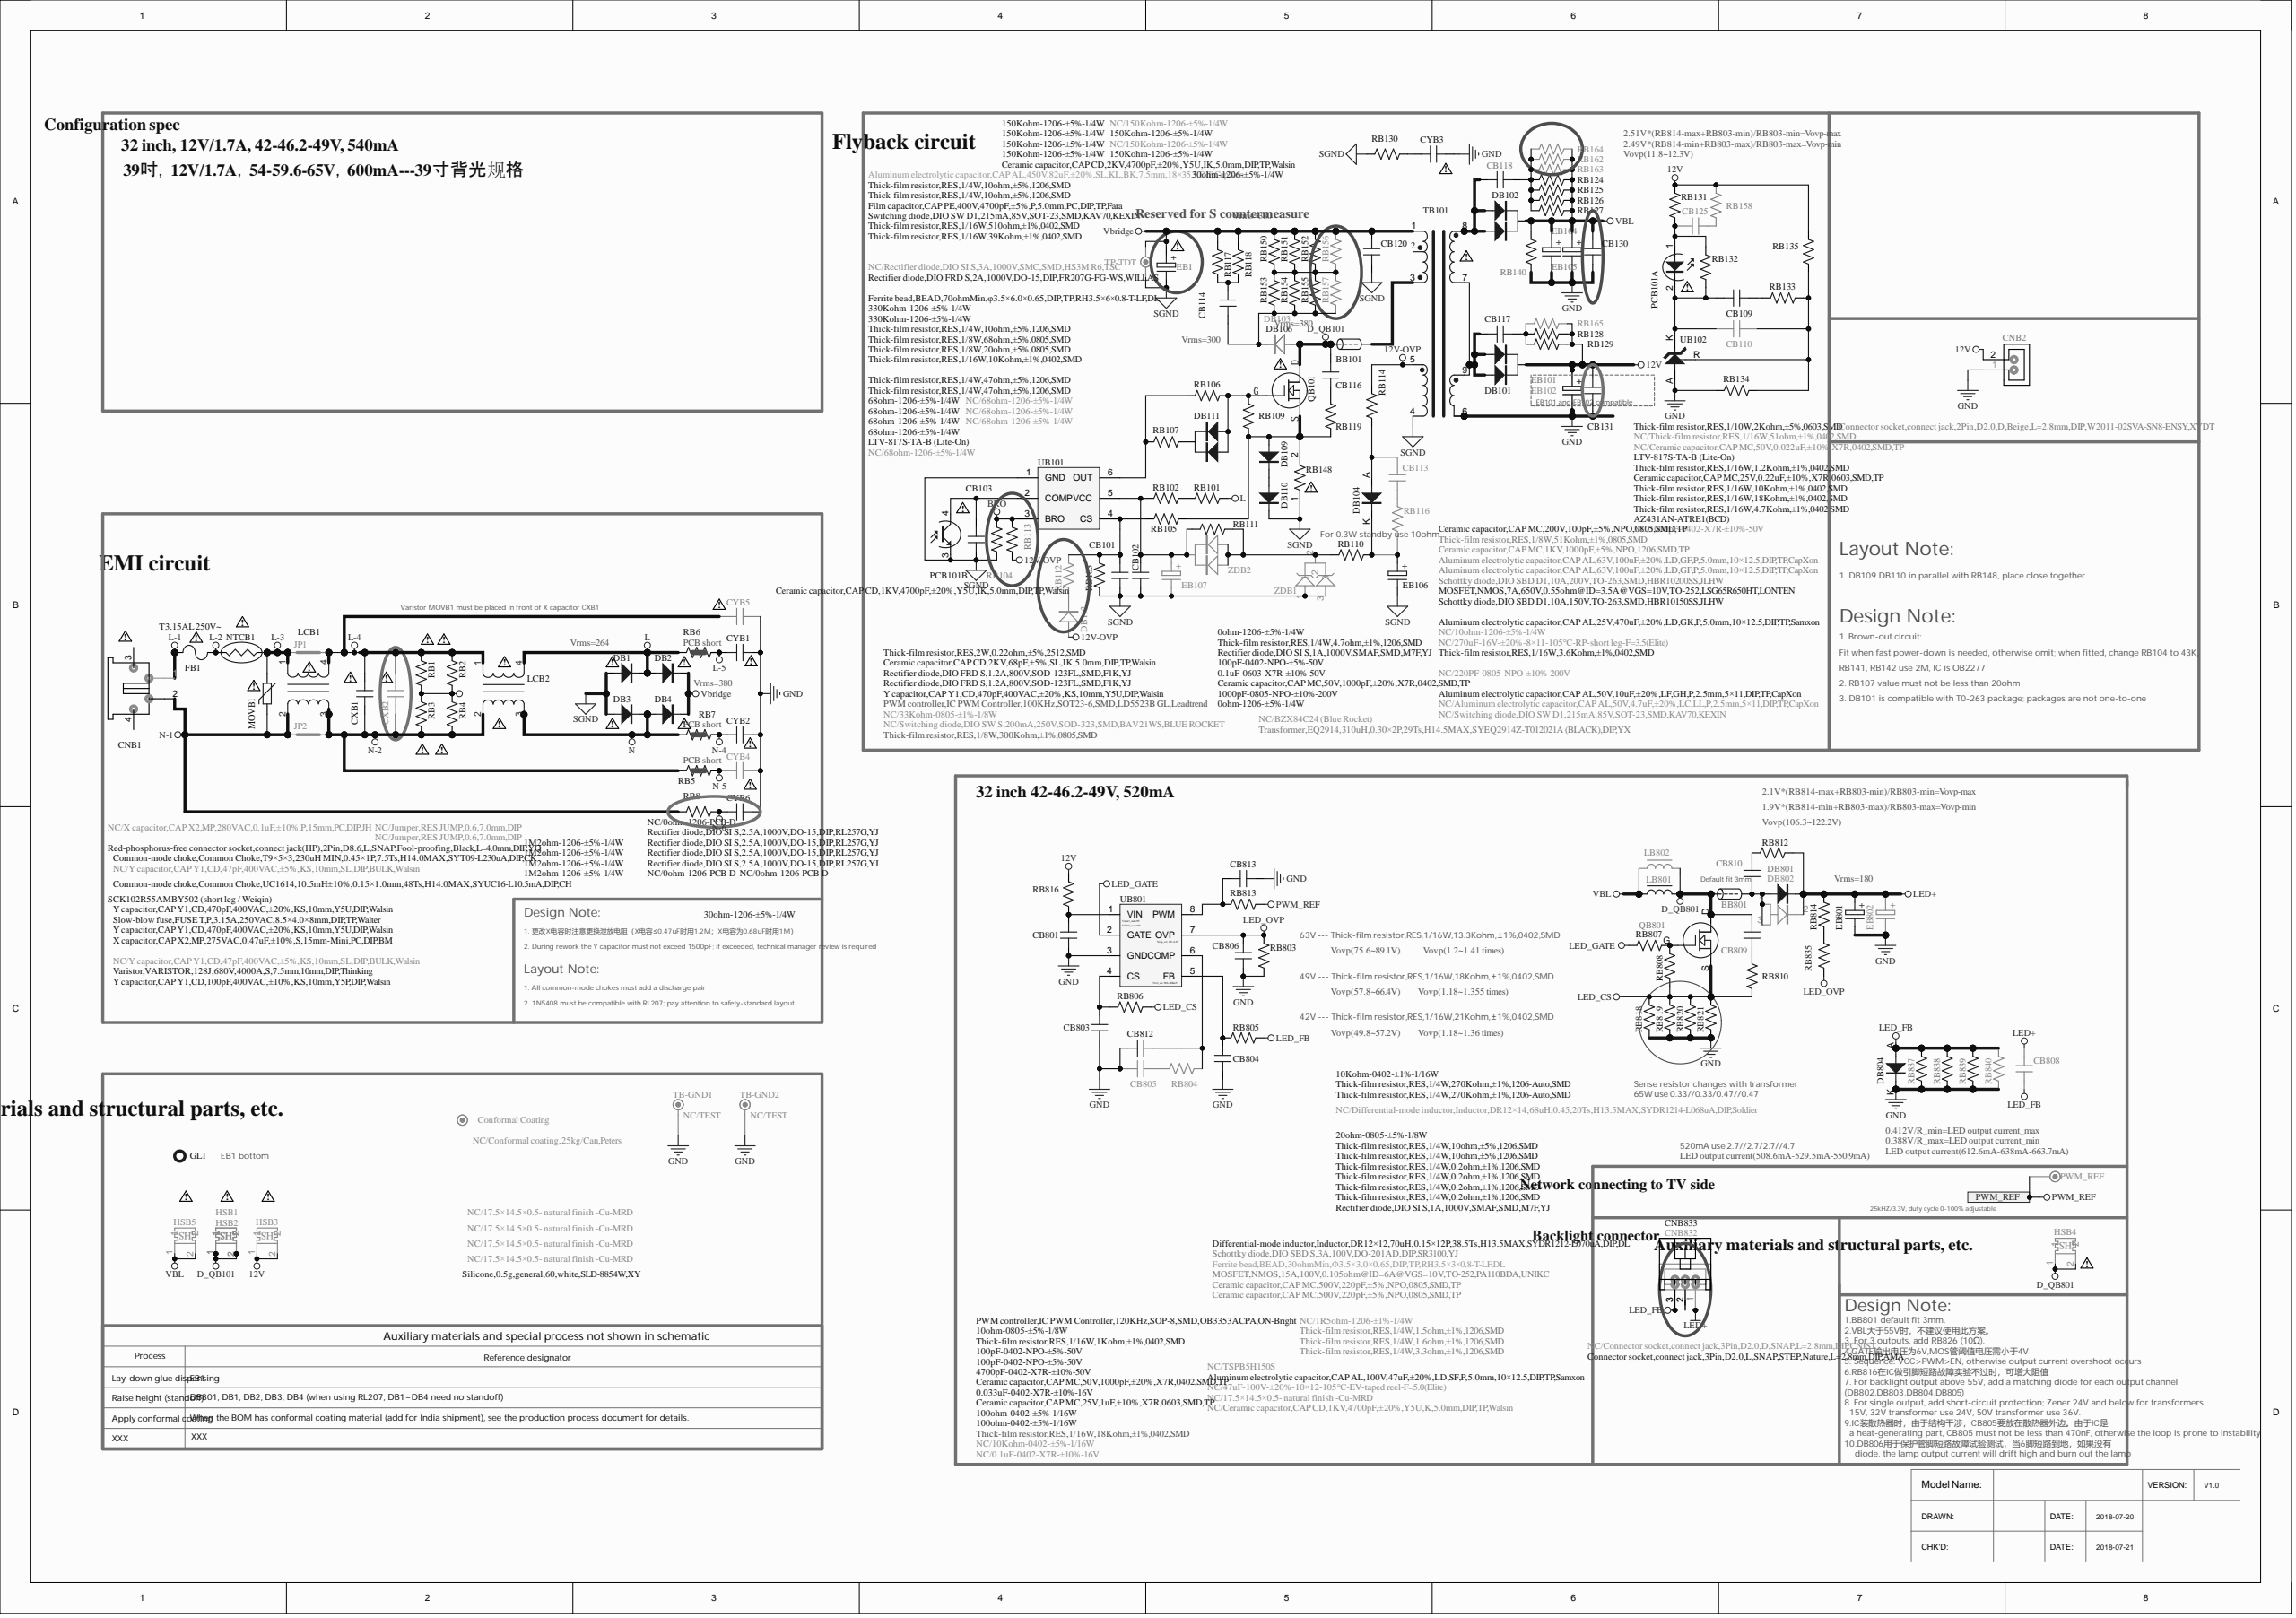Circuit board | Altium Designer | 574 parts | 274 nets | one sheet of the schematic
Parts on this sheet (reference | value | footprint):
BB101 | Ferrite bead,BEAD,70ohmMin,f3.5×6.0×0.65,DIP,TP,RH3.5×6×0.8-T-LF,DL | LB/3.5*6*12.5
BB801 | Ferrite bead,BEAD,30ohmMin,F3.5×3.0×0.65,DIP,TP,RH3.5×3×0.8-T-LF,DL | LB/3.5*6*12.5
CB101 | 100pF-0402-NPO-±5%-50V | C0402
CB102 | 0.1uF-0603-X7R-±10%-50V | C0603
CB103 | Ceramic capacitor,CAP MC,50V,1000pF,±20%,X7R,0402,SMD,TP | C0402
CB109 | Ceramic capacitor,CAP MC,25V,0.22uF,±10%,X7R,0603,SMD,TP | C0603
CB110 | NC/1000pF-0402-X7R-±10%-50V | C0402
CB113 | NC/220PF-0805-NPO-±10%-200V | C0805
CB114 | Film capacitor,CAP PE,400V,4700pF,±5%,P,5.0mm,PC,DIP,TP,Fara | CAP8*2.5-V-5
CB116 | Ceramic capacitor,CAP CD,2KV,68pF,±5%,SL,IK,5.0mm,DIP,TP,Walsin | CAP6.5*5-V-5-1
CB117 | 1000pF-0805-NPO-±10%-200V | C0805
CB118 | Ceramic capacitor,CAP MC,1KV,1000pF,±5%,NPO,1206,SMD,TP | C1206
CB120 | Ceramic capacitor,CAP CD,2KV,4700pF,±20%,Y5U,IK,5.0mm,DIP,TP,Walsin | CAP10*4.5-V-5
CB125 | NC/Ceramic capacitor,CAP MC,50V,0.022uF,±10%,X7R,0402,SMD,TP | C0402
CB130 | Ceramic capacitor,CAP CD,1KV,4700pF,±20%,Y5U,IK,5.0mm,DIP,TP,Walsin | CAP10*4.5-V-5
CB131 | Ceramic capacitor,CAP MC,200V,100pF,±5%,NPO,0805,SMD,TP | C0805
CB801 | Ceramic capacitor,CAP MC,25V,1uF,±10%,X7R,0603,SMD,TP | C0603
CB803 | 100pF-0402-NPO-±5%-50V | C0402
CB804 | 4700pF-0402-X7R-±10%-50V | C0402
CB805 | NC/0.1uF-0402-X7R-±10%-16V | C0402
CB806 | Ceramic capacitor,CAP MC,50V,1000pF,±20%,X7R,0402,SMD,TP | C0402
CB808 | NC/Ceramic capacitor,CAP CD,1KV,4700pF,±20%,Y5U,K,5.0mm,DIP,TP,Walsin | CAP10*4.5-V-5
CB809 | Ceramic capacitor,CAP MC,500V,220pF,±5%,NPO,0805,SMD,TP | C0805
CB810 | Ceramic capacitor,CAP MC,500V,220pF,±5%,NPO,0805,SMD,TP | C0805
CB812 | 0.033uF-0402-X7R-±10%-16V | C0402
CB813 | 100pF-0402-NPO-±5%-50V | C0402
CNB1 | Red-phosphorus-free connector socket,connect jack(HP),2Pin,D8.6,L,SNAP,Fool-proofing,Black,L=4.0mm,DIP,YQ | CON2-H8.6-1
CNB2 | Connector socket,connect jack,2Pin,D2.0,D,Beige,L=2.8mm,DIP,W2011-02SVA-SN8-ENSY,XYDT | SIP2/2.0D-1
CNB832 | NC/Connector socket,connect jack,3Pin,D2.0,D,SNAP,L=2.8mm,DIP,CNJST | SIP3/2.0D-CP
CNB833 | Connector socket,connect jack,3Pin,D2.0,L,SNAP,STEP,Nature,L=2.8mm,DIP,AMA | SIP3H/2.0D-3
CXB1 | X capacitor,CAP X2,MP,275VAC,0.47uF,±10%,S,15mm-Mini,PC,DIP,BM | CAP18*8.5-V-15
CXB2 | NC/X capacitor,CAP X2,MP,280VAC,0.1uF,±10%,P,15mm,PC,DIP,JH | CAP18*5*11.5-V-15
CYB1 | Y capacitor,CAP Y1,CD,470pF,400VAC,±20%,KS,10mm,Y5U,DIP,Walsin | CAP13*5-V-10-1
CYB2 | Y capacitor,CAP Y1,CD,470pF,400VAC,±20%,KS,10mm,Y5U,DIP,Walsin | CAP13*5-V-10-1
CYB3 | Y capacitor,CAP Y1,CD,470pF,400VAC,±20%,KS,10mm,Y5U,DIP,Walsin | CAP13*5-V-10-1
CYB4 | NC/Y capacitor,CAP Y1,CD,47pF,400VAC,±5%,KS,10mm,SL,DIP,BULK,Walsin | CAP13*5-V-10-1
CYB5 | NC/Y capacitor,CAP Y1,CD,47pF,400VAC,±5%,KS,10mm,SL,DIP,BULK,Walsin | CAP13*5-V-10-1
CYB6 | Y capacitor,CAP Y1,CD,100pF,400VAC,±10%,KS,10mm,Y5P,DIP,Walsin | CAP13*5-V-10-1
DB1 | Rectifier diode,DIO SI S,2.5A,1000V,DO-15,DIP,RL257G,YJ | D2-H-15
DB2 | Rectifier diode,DIO SI S,2.5A,1000V,DO-15,DIP,RL257G,YJ | D2-H-15
DB3 | Rectifier diode,DIO SI S,2.5A,1000V,DO-15,DIP,RL257G,YJ | D2-H-15
DB4 | Rectifier diode,DIO SI S,2.5A,1000V,DO-15,DIP,RL257G,YJ | D2-H-15
DB101 | Schottky diode,DIO SBD D1,10A,150V,TO-263,SMD,HBR10150SS,JLHW | D2PAK3
DB102 | Schottky diode,DIO SBD D1,10A,200V,TO-263,SMD,HBR10200SS,JLHW | D2PAK3
DB103 | NC/Rectifier diode,DIO SI S,3A,1000V,SMC,SMD,HS3M R6,TSC | DIODE-SMC
DB104 | Rectifier diode,DIO SI S,1A,1000V,SMAF,SMD,M7F,YJ | DIODE-S-2
DB106 | Rectifier diode,DIO FRD S,2A,1000V,DO-15,DIP,FR207G-FG-WS,WILLAS | D2-H-15
DB109 | Rectifier diode,DIO FRD S,1.2A,800V,SOD-123FL,SMD,F1K,YJ | DIODE-S-14
DB110 | Rectifier diode,DIO FRD S,1.2A,800V,SOD-123FL,SMD,F1K,YJ | DIODE-S-14
DB111 | Switching diode,DIO SW D1,215mA,85V,SOT-23,SMD,KAV70,KEXIN | SO-23
DB112 | NC/Switching diode,DIO SW S,200mA,250V,SOD-323,SMD,BAV21WS,BLUE ROCKET | DIODE-S-12
DB801 | Schottky diode,DIO SBD S,3A,100V,DO-201AD,DIP,SR3100,YJ | D3-H-20-2
DB802 | NC/TSPB5H150S | DIODE-S-13
DB804 | Rectifier diode,DIO SI S,1A,1000V,SMAF,SMD,M7F,YJ | DIODE-S-2
EB1 | Aluminum electrolytic capacitor,CAP AL,450V,82uF,±20%,SL,KL,BK,7.5mm,18×35.5,DIP,CapXon | EC(18*41)-H-7.5-1
EB101 | Aluminum electrolytic capacitor,CAP AL,25V,470uF,±20%,LD,GK,P,5.0mm,10×12.5,DIP,TP,Samxon | EC(10*12.5)-V-5
EB102 | NC/270uF-16V-±20%-8×11-105℃-RP-short leg-F=3.5(Elite) | EC(8*11)-V-3.5
EB105 | Aluminum electrolytic capacitor,CAP AL,63V,100uF,±20%,LD,GF,P,5.0mm,10×12.5,DIP,TP,CapXon | EC(10*12.5)-V-5
EB106 | Aluminum electrolytic capacitor,CAP AL,50V,10uF,±20%,LF,GH,P,2.5mm,5×11,DIP,TP,CapXon | EC(5*11)-V-2.5
EB107 | NC/Aluminum electrolytic capacitor,CAP AL,50V,4.7uF,±20%,LC,LL,P,2.5mm,5×11,DIP,TP,CapXon | EC(5*11)-V-2.5
EB801 | Aluminum electrolytic capacitor,CAP AL,100V,47uF,±20%,LD,SF,P,5.0mm,10×12.5,DIP,TP,Samxon | EC(10*12.5)-V-5
EB802 | NC/47uF-100V-±20%-10×12-105℃-EV-taped reel-F=5.0(Elite) | EC(10*12.5)-V-5
FB1 | Slow-blow fuse,FUSE T,P,3.15A,250VAC,8.5×4.0×8mm,DIP,TP,Walter | FUSE8.5*4-V-5(T3.15AL 250V~)
GL1 | Silicone,0.5g,general,60,white,SLD-8854W,XY | Silica gel-20
HSB1 | NC/17.5×14.5×0.5- natural finish -Cu-MRD | HS038
HSB2 | NC/17.5×14.5×0.5- natural finish -Cu-MRD | HS038
HSB3 | NC/17.5×14.5×0.5- natural finish -Cu-MRD | HS038
HSB4 | NC/17.5×14.5×0.5- natural finish -Cu-MRD | HS038
HSB5 | NC/17.5×14.5×0.5- natural finish -Cu-MRD | HS038
JP1 | NC/Jumper,RES JUMP,0.6,7.0mm,DIP | JP7.0
JP2 | NC/Jumper,RES JUMP,0.6,7.0mm,DIP | JP7.0
LB801 | Differential-mode inductor,Inductor,DR12×12,70uH,0.15×12P,38.5Ts,H13.5MAX,SYDR1212-L070uA,DIP,DL | L/LC2/15*14.5-V7.5
LB802 | NC/Differential-mode inductor,Inductor,DR12×14,68uH,0.45,20Ts,H13.5MAX,SYDR1214-L068uA,DIP,Soldier | L(13.5*15.5)-V-5
LCB1 | Common-mode choke,Common Choke,T9×5×3,230uH MIN,0.45×1P,7.5Ts,H14.0MAX,SYT09-L230uA,DIP,CK | L/LC4/12.8*10-V-6*7
LCB2 | Common-mode choke,Common Choke,UC1614,10.5mH±10%,0.15×1.0mm,48Ts,H14.0MAX,SYUC16-L10.5mA,DIP,CH | L/LC4/21*17-H-17*13
MOVB1 | Varistor,VARISTOR,128J,680V,4000A,S,7.5mm,10mm,DIP,Thinking | VR(13*5)-V-7.5
NTCB1 | SCK102R55AMBY502 (short leg / Weiqin) | NTC(10*5)-V5
PWM_REF | NC/TEST | TP_BL
QB101 | MOSFET,NMOS,7A,650V,0.55ohm@ID=3.5A@VGS=10V,TO-252,LSG65R650HT,LONTEN | D2PAK3
QB801 | MOSFET,NMOS,15A,100V,0.105ohm@ID=6A@VGS=10V,TO-252,PA110BDA,UNIKC | TO-252-GDS
RB1 | 1M2ohm-1206-±5%-1/4W | R1206
RB2 | 1M2ohm-1206-±5%-1/4W | R1206
RB3 | 1M2ohm-1206-±5%-1/4W | R1206
RB4 | 1M2ohm-1206-±5%-1/4W | R1206
RB5 | NC/0ohm-1206-PCB-D | R1206SC
RB6 | NC/0ohm-1206-PCB-D | R1206SC
RB7 | NC/0ohm-1206-PCB-D | R1206SC
RB8 | 30ohm-1206-±5%-1/4W | R1206
RB101 | 330Kohm-1206-±5%-1/4W | R1206
RB102 | 330Kohm-1206-±5%-1/4W | R1206
RB103 | Thick-film resistor,RES,1/16W,3.6Kohm,±1%,0402,SMD | R0402
RB104 | Thick-film resistor,RES,1/16W,39Kohm,±1%,0402,SMD | R0402
RB105 | Thick-film resistor,RES,1/16W,510ohm,±1%,0402,SMD | R0402
RB106 | Thick-film resistor,RES,1/8W,68ohm,±5%,0805,SMD | R0805
RB107 | Thick-film resistor,RES,1/8W,20ohm,±5%,0805,SMD | R0805
RB109 | Thick-film resistor,RES,1/16W,10Kohm,±1%,0402,SMD | R0402
RB110 | 0ohm-1206-±5%-1/4W | R1206
RB111 | 0ohm-1206-±5%-1/4W | R1206
RB112 | NC/33Kohm-0805-±1%-1/8W | R0805
RB113 | Thick-film resistor,RES,1/8W,300Kohm,±1%,0805,SMD | R0805
RB114 | Thick-film resistor,RES,1/4W,4.7ohm,±1%,1206,SMD | R1206
RB116 | NC/10ohm-1206-±5%-1/4W | R1206
RB117 | Thick-film resistor,RES,1/4W,10ohm,±5%,1206,SMD | R1206
RB118 | Thick-film resistor,RES,1/4W,10ohm,±5%,1206,SMD | R1206
RB119 | Thick-film resistor,RES,1/4W,10ohm,±5%,1206,SMD | R1206
RB124 | 68ohm-1206-±5%-1/4W | R1206
RB125 | 68ohm-1206-±5%-1/4W | R1206
RB126 | 68ohm-1206-±5%-1/4W | R1206
RB127 | 68ohm-1206-±5%-1/4W | R1206
RB128 | Thick-film resistor,RES,1/4W,47ohm,±5%,1206,SMD | R1206
RB129 | Thick-film resistor,RES,1/4W,47ohm,±5%,1206,SMD | R1206
RB130 | 30ohm-1206-±5%-1/4W | R1206
RB131 | Thick-film resistor,RES,1/10W,2Kohm,±5%,0603,SMD | R0603
RB132 | Thick-film resistor,RES,1/16W,1.2Kohm,±1%,0402,SMD | R0402
RB133 | Thick-film resistor,RES,1/16W,10Kohm,±1%,0402,SMD | R0402
RB134 | Thick-film resistor,RES,1/16W,4.7Kohm,±1%,0402,SMD | R0402
RB135 | Thick-film resistor,RES,1/16W,18Kohm,±1%,0402,SMD | R0402
RB140 | Thick-film resistor,RES,1/8W,51Kohm,±1%,0805,SMD | R0805
RB148 | Thick-film resistor,RES,2W,0.22ohm,±5%,2512,SMD | R2512-1
RB150 | 150Kohm-1206-±5%-1/4W | R1206
RB151 | 150Kohm-1206-±5%-1/4W | R1206
RB152 | 150Kohm-1206-±5%-1/4W | R1206
RB153 | 150Kohm-1206-±5%-1/4W | R1206
RB154 | 150Kohm-1206-±5%-1/4W | R1206
RB155 | 150Kohm-1206-±5%-1/4W | R1206
RB156 | NC/150Kohm-1206-±5%-1/4W | R1206
RB157 | NC/150Kohm-1206-±5%-1/4W | R1206
RB158 | NC/Thick-film resistor,RES,1/16W,51ohm,±1%,0402,SMD | R0402
RB162 | NC/68ohm-1206-±5%-1/4W | R1206
RB163 | NC/68ohm-1206-±5%-1/4W | R1206
RB164 | NC/68ohm-1206-±5%-1/4W | R1206
RB165 | NC/68ohm-1206-±5%-1/4W | R1206
RB803 | Thick-film resistor,RES,1/16W,18Kohm,±1%,0402,SMD | R0402
RB804 | NC/10Kohm-0402-±5%-1/16W | R0402
RB805 | 100ohm-0402-±5%-1/16W | R0402
RB806 | Thick-film resistor,RES,1/16W,1Kohm,±1%,0402,SMD | R0402
RB807 | 20ohm-0805-±5%-1/8W | R0805
RB808 | 10Kohm-0402-±1%-1/16W | R0402
RB810 | Thick-film resistor,RES,1/4W,10ohm,±5%,1206,SMD | R1206
RB812 | Thick-film resistor,RES,1/4W,10ohm,±5%,1206,SMD | R1206
RB813 | 100ohm-0402-±5%-1/16W | R0402
RB814 | Thick-film resistor,RES,1/4W,270Kohm,±1%,1206-Auto,SMD | R1206
RB816 | 10ohm-0805-±5%-1/8W | R0805
RB818 | Thick-film resistor,RES,1/4W,0.2ohm,±1%,1206,SMD | R1206
RB819 | Thick-film resistor,RES,1/4W,0.2ohm,±1%,1206,SMD | R1206
RB820 | Thick-film resistor,RES,1/4W,0.2ohm,±1%,1206,SMD | R1206
RB821 | Thick-film resistor,RES,1/4W,0.2ohm,±1%,1206,SMD | R1206
RB835 | Thick-film resistor,RES,1/4W,270Kohm,±1%,1206-Auto,SMD | R1206
RB837 | Thick-film resistor,RES,1/4W,1.5ohm,±1%,1206,SMD | R1206
RB838 | Thick-film resistor,RES,1/4W,1.6ohm,±1%,1206,SMD | R1206
RB839 | Thick-film resistor,RES,1/4W,3.3ohm,±1%,1206,SMD | R1206
RB840 | NC/1R5ohm-1206-±1%-1/4W | R1206
TB101 | Transformer,EQ2914,310uH,0.30×2P,29Ts,H14.5MAX,SYEQ2914Z-T012021A (BLACK),DIP,YX | T/EQ2914*9-1
TB-GND1 | NC/TEST | TP-10
TB-GND2 | NC/TEST | TP-10
TP-TDT | NC/ | TP-TDT
UB101 | PWM controller,IC PWM Controller,100KHz,SOT23-6,SMD,LD5523B GL,Leadtrend | SOT-26
UB102 | AZ431AN-ATRE1(BCD) | SOT-23-RAK
UB801 | PWM controller,IC PWM Controller,120KHz,SOP-8,SMD,OB3353ACPA,ON-Bright | SO-8A
ZDB1 | NC/BZX84C24 (Blue Rocket) | SO-23
ZDB2 | NC/Switching diode,DIO SW D1,215mA,85V,SOT-23,SMD,KAV70,KEXIN | SO-23
Nets of these parts (net: part-pin ...):
Vbridge: CB120-2 DB2-K DB4-K EB1-1 RB117-2 RB118-2 RB150-2 RB151-2 RB152-2 RB156-2 TB101-1 TP-TDT-1
VBL: CB130-2 DB102-2 EB105-1 HSB5-1 HSB5-2 LB801-1 LB802-1 RB124-2 RB125-2 RB126-2 RB127-2 RB140-1 RB162-2 RB163-2 RB164-2
SGND: CB101-2 CB102-2 CB103-2 CB120-1 DB1-A DB3-A DB110-K EB1-2 EB106-2 EB107-2 RB103-1 RB104-1 RB130-1 RB148-1 TB101-4 TP-TDT-2 UB101-1 ZDB1-1 ZDB1-3
PWM_REF: PWM_REF-1 RB813-2
NetRB814_2: RB814-2 RB835-1
NetRB150_1: RB150-1 RB151-1 RB152-1 RB153-2 RB154-2 RB155-2 RB156-1 RB157-2
NetRB110_1: RB110-1 RB111-2 ZDB1-2 ZDB2-1 ZDB2-3
NetRB106_1: RB106-1 RB107-1 UB101-6
NetRB101_2: RB101-2 RB102-1
NetQB801_G: QB801-G RB807-2 RB808-2
NetDB112_K: DB112-K RB112-2
NetDB111_2: DB111-2 RB107-2
NetDB111_1: DB111-1 DB111-3 QB101-1 RB106-2 RB109-2
NetDB109_K: DB109-K DB110-A
NetDB109_A: DB109-A QB101-3 RB105-2 RB109-1 RB119-1 RB148-2
NetDB104_K: DB104-K EB106-1 RB110-2 RB116-2
NetCYB3_1: CYB3-1 RB130-2
NetCNB832_2: CNB832-2 CNB833-2
NetCB813_2: CB813-2 RB813-1 UB801-8
NetCB812_2: CB812-2 RB804-2 UB801-6
NetCB810_2: CB810-2 RB812-1
NetCB809_1: CB809-1 RB810-1
NetCB805_2: CB805-2 RB804-1
NetCB804_1: CB804-1 RB805-1 UB801-5
NetCB803_1: CB803-1 RB806-1 UB801-4
NetCB801_2: CB801-2 RB816-2 UB801-1
NetCB125_2: CB125-2 RB158-1
NetCB125_1: CB125-1 RB131-1 RB132-2
NetCB118_2: CB118-2 RB124-1 RB125-1 RB126-1 RB127-1 RB162-1 RB163-1 RB164-1
NetCB118_1: CB118-1 DB102-1 DB102-3 TB101-8
NetCB117_2: CB117-2 RB128-1 RB129-1 RB165-1
NetCB117_1: CB117-1 DB101-1 DB101-3 TB101-7 TB101-9
NetCB116_1: CB116-1 RB119-2
NetCB114_2: CB114-2 DB103-K DB106-K RB153-1 RB154-1 RB155-1 RB157-1
NetCB114_1: CB114-1 RB117-1 RB118-1
NetCB113_2: CB113-2 RB116-1
NetCB113_1: CB113-1 DB104-A RB114-1
NetCB110_2: CB110-2 RB133-1 RB134-2 RB135-2 UB102-R
NetCB109_2: CB109-2 RB133-2
NetCB109_1: CB109-1 CB110-1 RB132-1 UB102-K
NetCB103_1: CB103-1 UB101-2
NetCB102_1: CB102-1 EB107-1 RB102-2 RB111-1 UB101-5 ZDB2-2
NetCB101_1: CB101-1 RB103-2 RB105-1 RB112-1 UB101-4
NetBB801_2: BB801-2 CB810-1 DB801-A DB802-1 DB802-3
NetBB101_2: BB101-2 TB101-3
N-6: CYB6-1 RB8-2
N-5: CYB4-1 RB5-2 RB5-3
N-4: CYB2-1 RB7-2 RB7-3
N-2: CXB1-2 CXB2-1 JP2-1 LCB1-3 LCB2-2 RB3-2 RB4-2 RB5-1
N-1: CNB1-2 JP2-2 LCB1-2 MOVB1-2 RB8-1
N: DB3-K DB4-A LCB2-3 RB7-1
LED_OVP: CB806-1 RB803-2 RB835-2 UB801-7
LED_GATE: RB807-1 UB801-2
LED_FB: CB808-1 CNB832-3 CNB833-3 DB804-A RB805-2 RB837-2 RB838-2 RB839-1 RB840-2
LED_CS: QB801-S RB806-2 RB808-1 RB810-2 RB818-1 RB819-1 RB820-1 RB821-1
LED+: CB808-2 CNB832-1 CNB833-1 DB801-K DB802-2 EB801-1 EB802-1 RB812-2 RB814-1
L-N: RB1-2 RB2-2 RB3-1 RB4-1
L-5: CYB1-1 RB6-2 RB6-3
L-4: CXB1-1 CXB2-2 CYB5-1 JP1-1 LCB1-4 LCB2-1 RB1-1 RB2-1
L-3: JP1-2 LCB1-1 MOVB1-1 NTCB1-1
L-2: FB1-2 NTCB1-2
L-1: CNB1-1 FB1-1
L: DB1-K DB2-A LCB2-4 RB6-1 RB101-1
GND: CB130-1 CB131-2 CB801-1 CB803-2 CB804-2 CB805-1 CB806-2 CB812-1 CB813-1 CNB2-1 CYB1-2 CYB2-2 CYB3-2 CYB4-2 CYB5-2 CYB6-2 DB804-K EB101-2 EB102-2 EB105-2 EB801-2 EB802-2 RB134-1 RB140-2 RB803-1 RB818-2 RB819-2 RB820-2 RB821-2 RB837-1 RB838-1 RB839-2 RB840-1 TB101-6 TB-GND1-1 TB-GND2-1 UB102-A UB801-3
D_QB801: BB801-1 CB809-2 HSB4-1 HSB4-2 LB801-2 LB802-2 QB801-D
D_QB101: BB101-1 CB116-2 DB103-A DB106-A HSB1-1 HSB1-2 HSB2-1 HSB2-2 QB101-2
BRO: RB104-2 RB113-1 UB101-3
12V-OVP: DB112-A RB113-2 RB114-2 TB101-5
12V: CB131-1 CNB2-2 DB101-2 EB101-1 EB102-1 HSB3-1 HSB3-2 RB128-2 RB129-2 RB131-2 RB135-1 RB158-2 RB165-2 RB816-1